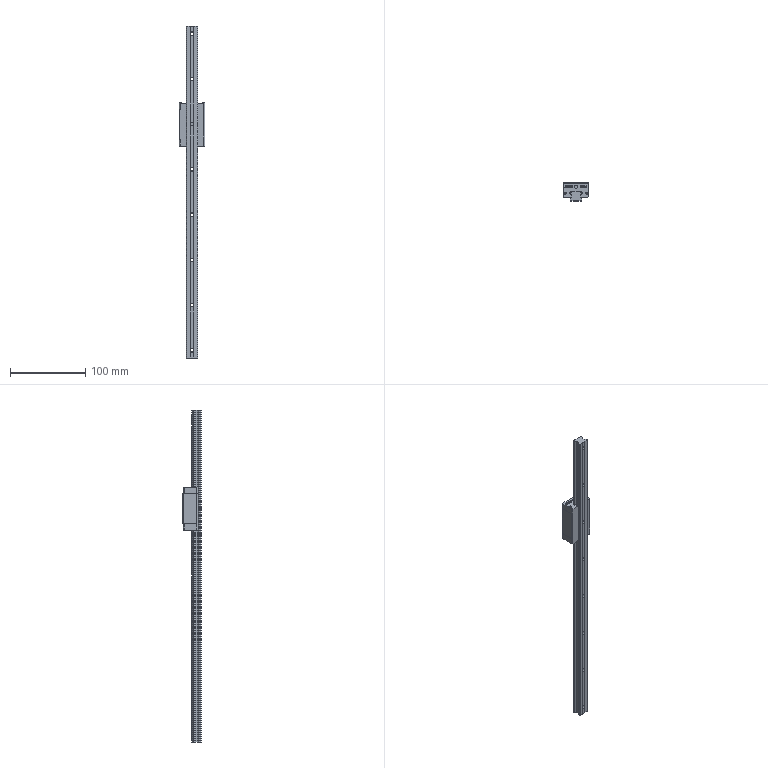Part | SolidWorks | 2 solids | 484 faces | box 34 x 24 x 440 mm | volume 99523 mm3 | plane 301 | cylinder 115 | spline 68 | commonest cylinder face diameters 1.6 x16 4.5 x16 8 x16 0.6 x15 2.1 x12 4 x12